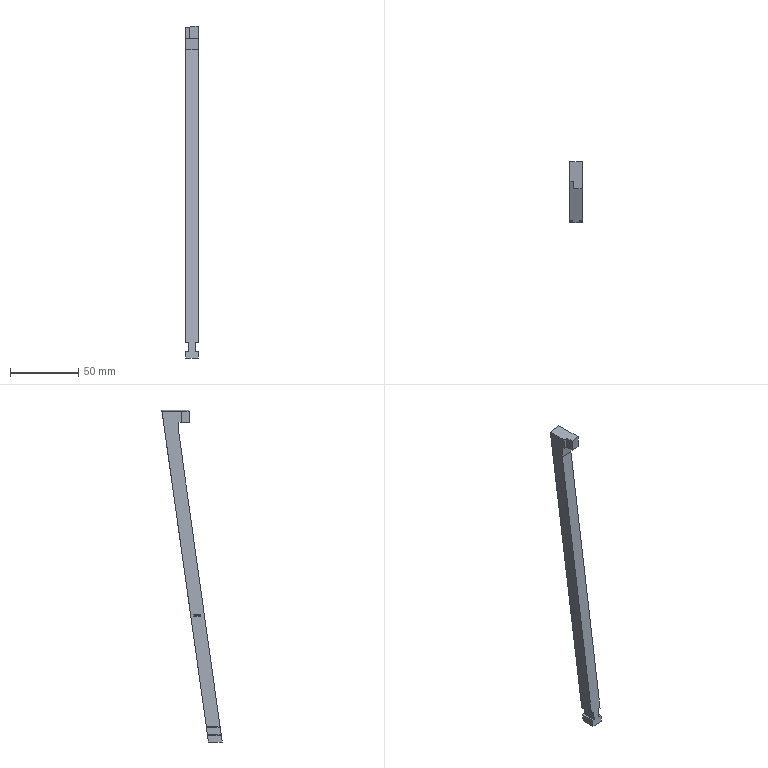Part | Creo | 1 solid | 98 faces | box 9 x 44.327 x 243.554 mm | volume 22449 mm3 | other 55 | plane 38 | cylinder 5 | commonest cylinder face diameters 1 x4 19.132 x1